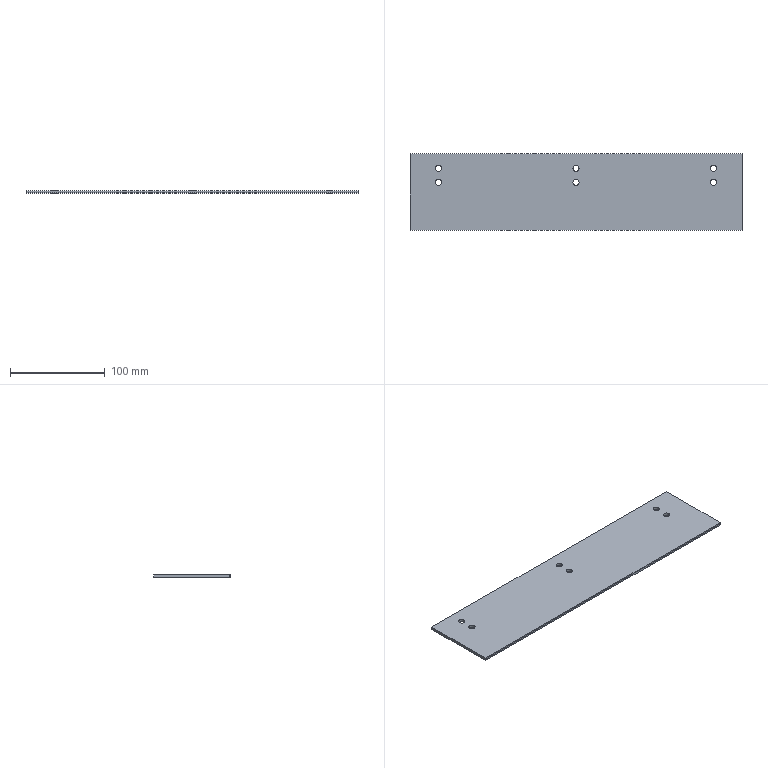Part | SolidWorks | features Extrusion 1, ICE 1 | 1 solid | 19 faces | box 350 x 80.217 x 3 mm | volume 83584 mm3 | cylinder 14 | plane 5 | commonest cylinder face diameters 6.5 x12 33.7 x2
STEP:
#1=CARTESIAN_POINT('',(-175.,-37.65,1.5));
#2=VERTEX_POINT('',#1);
#3=CARTESIAN_POINT('',(-175.,-37.717,3.));
#4=VERTEX_POINT('',#3);
#5=CARTESIAN_POINT('',(-175.,-54.5,1.5));
#6=DIRECTION('',(1.,0.,0.));
#7=DIRECTION('',(0.,0.,-1.));
#8=AXIS2_PLACEMENT_3D('',#5,#6,#7);
#9=CIRCLE('',#8,16.85);
#10=EDGE_CURVE('',#2,#4,#9,.T.);
#11=ORIENTED_EDGE('',*,*,#10,.F.);
#12=CARTESIAN_POINT('',(175.,-37.65,1.5));
#13=VERTEX_POINT('',#12);
#14=CARTESIAN_POINT('',(-191.,-37.65,1.5));
#15=DIRECTION('',(1.,0.,0.));
#16=VECTOR('',#15,1000.);
#17=LINE('',#14,#16);
#18=EDGE_CURVE('',#2,#13,#17,.T.);
#19=ORIENTED_EDGE('',*,*,#18,.T.);
#20=CARTESIAN_POINT('',(175.,-37.717,3.));
#21=VERTEX_POINT('',#20);
#22=CARTESIAN_POINT('',(175.,-54.5,1.5));
#23=DIRECTION('',(1.,0.,0.));
#24=DIRECTION('',(0.,1.,0.));
#25=AXIS2_PLACEMENT_3D('',#22,#23,#24);
#26=CIRCLE('',#25,16.85);
#27=EDGE_CURVE('',#13,#21,#26,.T.);
#28=ORIENTED_EDGE('',*,*,#27,.T.);
#29=CARTESIAN_POINT('',(-191.,-37.717,3.));
#30=DIRECTION('',(-1.,0.,0.));
#31=VECTOR('',#30,1000.);
#32=LINE('',#29,#31);
#33=EDGE_CURVE('',#21,#4,#32,.T.);
#34=ORIENTED_EDGE('',*,*,#33,.T.);
#35=EDGE_LOOP('',(#11,#19,#28,#34));
#36=FACE_OUTER_BOUND('',#35,.T.);
#37=CARTESIAN_POINT('',(-191.,-54.5,1.5));
#38=DIRECTION('',(1.,0.,0.));
#39=DIRECTION('',(0.,1.,0.));
#40=AXIS2_PLACEMENT_3D('',#37,#38,#39);
#41=CYLINDRICAL_SURFACE('',#40,16.85);
#42=ADVANCED_FACE('',(#36),#41,.F.);
#43=CARTESIAN_POINT('',(141.75,12.5,3.));
#44=VERTEX_POINT('',#43);
#45=CARTESIAN_POINT('',(148.25,12.5,3.));
#46=VERTEX_POINT('',#45);
#47=CARTESIAN_POINT('',(145.,12.5,3.));
#48=DIRECTION('',(0.,0.,1.));
#49=DIRECTION('',(1.,0.,0.));
#50=AXIS2_PLACEMENT_3D('',#47,#48,#49);
#51=CIRCLE('',#50,3.25);
#52=EDGE_CURVE('',#44,#46,#51,.T.);
#53=ORIENTED_EDGE('',*,*,#52,.T.);
#54=CARTESIAN_POINT('',(148.25,12.5,0.));
#55=VERTEX_POINT('',#54);
#56=CARTESIAN_POINT('',(148.25,12.5,3.));
#57=DIRECTION('',(0.,0.,-1.));
#58=VECTOR('',#57,1000.);
#59=LINE('',#56,#58);
#60=EDGE_CURVE('',#46,#55,#59,.T.);
#61=ORIENTED_EDGE('',*,*,#60,.T.);
#62=CARTESIAN_POINT('',(141.75,12.5,0.));
#63=VERTEX_POINT('',#62);
#64=CARTESIAN_POINT('',(145.,12.5,0.));
#65=DIRECTION('',(0.,0.,1.));
#66=DIRECTION('',(1.,0.,0.));
#67=AXIS2_PLACEMENT_3D('',#64,#65,#66);
#68=CIRCLE('',#67,3.25);
#69=EDGE_CURVE('',#63,#55,#68,.T.);
#70=ORIENTED_EDGE('',*,*,#69,.F.);
#71=CARTESIAN_POINT('',(141.75,12.5,3.));
#72=DIRECTION('',(0.,0.,-1.));
#73=VECTOR('',#72,1000.);
#74=LINE('',#71,#73);
#75=EDGE_CURVE('',#44,#63,#74,.T.);
#76=ORIENTED_EDGE('',*,*,#75,.F.);
#77=EDGE_LOOP('',(#53,#61,#70,#76));
#78=FACE_OUTER_BOUND('',#77,.T.);
#79=CARTESIAN_POINT('',(145.,12.5,3.));
#80=DIRECTION('',(0.,0.,-1.));
#81=DIRECTION('',(-1.,0.,0.));
#82=AXIS2_PLACEMENT_3D('',#79,#80,#81);
#83=CYLINDRICAL_SURFACE('',#82,3.25);
#84=ADVANCED_FACE('',(#78),#83,.F.);
#85=CARTESIAN_POINT('',(141.75,27.5,3.));
#86=VERTEX_POINT('',#85);
#87=CARTESIAN_POINT('',(148.25,27.5,3.));
#88=VERTEX_POINT('',#87);
#89=CARTESIAN_POINT('',(145.,27.5,3.));
#90=DIRECTION('',(0.,0.,1.));
#91=DIRECTION('',(1.,0.,0.));
#92=AXIS2_PLACEMENT_3D('',#89,#90,#91);
#93=CIRCLE('',#92,3.25);
#94=EDGE_CURVE('',#86,#88,#93,.T.);
#95=ORIENTED_EDGE('',*,*,#94,.T.);
#96=CARTESIAN_POINT('',(148.25,27.5,0.));
#97=VERTEX_POINT('',#96);
#98=CARTESIAN_POINT('',(148.25,27.5,3.));
#99=DIRECTION('',(0.,0.,-1.));
#100=VECTOR('',#99,1000.);
#101=LINE('',#98,#100);
#102=EDGE_CURVE('',#88,#97,#101,.T.);
#103=ORIENTED_EDGE('',*,*,#102,.T.);
#104=CARTESIAN_POINT('',(141.75,27.5,0.));
#105=VERTEX_POINT('',#104);
#106=CARTESIAN_POINT('',(145.,27.5,0.));
#107=DIRECTION('',(0.,0.,1.));
#108=DIRECTION('',(1.,0.,0.));
#109=AXIS2_PLACEMENT_3D('',#106,#107,#108);
#110=CIRCLE('',#109,3.25);
#111=EDGE_CURVE('',#105,#97,#110,.T.);
#112=ORIENTED_EDGE('',*,*,#111,.F.);
#113=CARTESIAN_POINT('',(141.75,27.5,3.));
#114=DIRECTION('',(0.,0.,-1.));
#115=VECTOR('',#114,1000.);
#116=LINE('',#113,#115);
#117=EDGE_CURVE('',#86,#105,#116,.T.);
#118=ORIENTED_EDGE('',*,*,#117,.F.);
#119=EDGE_LOOP('',(#95,#103,#112,#118));
#120=FACE_OUTER_BOUND('',#119,.T.);
#121=CARTESIAN_POINT('',(145.,27.5,3.));
#122=DIRECTION('',(0.,0.,-1.));
#123=DIRECTION('',(-1.,0.,0.));
#124=AXIS2_PLACEMENT_3D('',#121,#122,#123);
#125=CYLINDRICAL_SURFACE('',#124,3.25);
#126=ADVANCED_FACE('',(#120),#125,.F.);
#127=CARTESIAN_POINT('',(-3.25,12.5,3.));
#128=VERTEX_POINT('',#127);
#129=CARTESIAN_POINT('',(3.25,12.5,3.));
#130=VERTEX_POINT('',#129);
#131=CARTESIAN_POINT('',(0.,12.5,3.));
#132=DIRECTION('',(0.,0.,1.));
#133=DIRECTION('',(1.,0.,0.));
#134=AXIS2_PLACEMENT_3D('',#131,#132,#133);
#135=CIRCLE('',#134,3.25);
#136=EDGE_CURVE('',#128,#130,#135,.T.);
#137=ORIENTED_EDGE('',*,*,#136,.T.);
#138=CARTESIAN_POINT('',(3.25,12.5,0.));
#139=VERTEX_POINT('',#138);
#140=CARTESIAN_POINT('',(3.25,12.5,3.));
#141=DIRECTION('',(0.,0.,-1.));
#142=VECTOR('',#141,1000.);
#143=LINE('',#140,#142);
#144=EDGE_CURVE('',#130,#139,#143,.T.);
#145=ORIENTED_EDGE('',*,*,#144,.T.);
#146=CARTESIAN_POINT('',(-3.25,12.5,0.));
#147=VERTEX_POINT('',#146);
#148=CARTESIAN_POINT('',(0.,12.5,0.));
#149=DIRECTION('',(0.,0.,1.));
#150=DIRECTION('',(1.,0.,0.));
#151=AXIS2_PLACEMENT_3D('',#148,#149,#150);
#152=CIRCLE('',#151,3.25);
#153=EDGE_CURVE('',#147,#139,#152,.T.);
#154=ORIENTED_EDGE('',*,*,#153,.F.);
#155=CARTESIAN_POINT('',(-3.25,12.5,3.));
#156=DIRECTION('',(0.,0.,-1.));
#157=VECTOR('',#156,1000.);
#158=LINE('',#155,#157);
#159=EDGE_CURVE('',#128,#147,#158,.T.);
#160=ORIENTED_EDGE('',*,*,#159,.F.);
#161=EDGE_LOOP('',(#137,#145,#154,#160));
#162=FACE_OUTER_BOUND('',#161,.T.);
#163=CARTESIAN_POINT('',(0.,12.5,3.));
#164=DIRECTION('',(0.,0.,-1.));
#165=DIRECTION('',(-1.,0.,0.));
#166=AXIS2_PLACEMENT_3D('',#163,#164,#165);
#167=CYLINDRICAL_SURFACE('',#166,3.25);
#168=ADVANCED_FACE('',(#162),#167,.F.);
#169=CARTESIAN_POINT('',(-3.25,27.5,3.));
#170=VERTEX_POINT('',#169);
#171=CARTESIAN_POINT('',(3.25,27.5,3.));
#172=VERTEX_POINT('',#171);
#173=CARTESIAN_POINT('',(0.,27.5,3.));
#174=DIRECTION('',(0.,0.,1.));
#175=DIRECTION('',(1.,0.,0.));
#176=AXIS2_PLACEMENT_3D('',#173,#174,#175);
#177=CIRCLE('',#176,3.25);
#178=EDGE_CURVE('',#170,#172,#177,.T.);
#179=ORIENTED_EDGE('',*,*,#178,.T.);
#180=CARTESIAN_POINT('',(3.25,27.5,0.));
#181=VERTEX_POINT('',#180);
#182=CARTESIAN_POINT('',(3.25,27.5,3.));
#183=DIRECTION('',(0.,0.,-1.));
#184=VECTOR('',#183,1000.);
#185=LINE('',#182,#184);
#186=EDGE_CURVE('',#172,#181,#185,.T.);
#187=ORIENTED_EDGE('',*,*,#186,.T.);
#188=CARTESIAN_POINT('',(-3.25,27.5,0.));
#189=VERTEX_POINT('',#188);
#190=CARTESIAN_POINT('',(0.,27.5,0.));
#191=DIRECTION('',(0.,0.,1.));
#192=DIRECTION('',(1.,0.,0.));
#193=AXIS2_PLACEMENT_3D('',#190,#191,#192);
#194=CIRCLE('',#193,3.25);
#195=EDGE_CURVE('',#189,#181,#194,.T.);
#196=ORIENTED_EDGE('',*,*,#195,.F.);
#197=CARTESIAN_POINT('',(-3.25,27.5,3.));
#198=DIRECTION('',(0.,0.,-1.));
#199=VECTOR('',#198,1000.);
#200=LINE('',#197,#199);
#201=EDGE_CURVE('',#170,#189,#200,.T.);
#202=ORIENTED_EDGE('',*,*,#201,.F.);
#203=EDGE_LOOP('',(#179,#187,#196,#202));
#204=FACE_OUTER_BOUND('',#203,.T.);
#205=CARTESIAN_POINT('',(0.,27.5,3.));
#206=DIRECTION('',(0.,0.,-1.));
#207=DIRECTION('',(-1.,0.,0.));
#208=AXIS2_PLACEMENT_3D('',#205,#206,#207);
#209=CYLINDRICAL_SURFACE('',#208,3.25);
#210=ADVANCED_FACE('',(#204),#209,.F.);
#211=CARTESIAN_POINT('',(-148.25,12.5,3.));
#212=VERTEX_POINT('',#211);
#213=CARTESIAN_POINT('',(-141.75,12.5,3.));
#214=VERTEX_POINT('',#213);
#215=CARTESIAN_POINT('',(-145.,12.5,3.));
#216=DIRECTION('',(0.,0.,1.));
#217=DIRECTION('',(1.,0.,0.));
#218=AXIS2_PLACEMENT_3D('',#215,#216,#217);
#219=CIRCLE('',#218,3.25);
#220=EDGE_CURVE('',#212,#214,#219,.T.);
#221=ORIENTED_EDGE('',*,*,#220,.T.);
#222=CARTESIAN_POINT('',(-141.75,12.5,0.));
#223=VERTEX_POINT('',#222);
#224=CARTESIAN_POINT('',(-141.75,12.5,3.));
#225=DIRECTION('',(0.,0.,-1.));
#226=VECTOR('',#225,1000.);
#227=LINE('',#224,#226);
#228=EDGE_CURVE('',#214,#223,#227,.T.);
#229=ORIENTED_EDGE('',*,*,#228,.T.);
#230=CARTESIAN_POINT('',(-148.25,12.5,0.));
#231=VERTEX_POINT('',#230);
#232=CARTESIAN_POINT('',(-145.,12.5,0.));
#233=DIRECTION('',(0.,0.,1.));
#234=DIRECTION('',(1.,0.,0.));
#235=AXIS2_PLACEMENT_3D('',#232,#233,#234);
#236=CIRCLE('',#235,3.25);
#237=EDGE_CURVE('',#231,#223,#236,.T.);
#238=ORIENTED_EDGE('',*,*,#237,.F.);
#239=CARTESIAN_POINT('',(-148.25,12.5,3.));
#240=DIRECTION('',(0.,0.,-1.));
#241=VECTOR('',#240,1000.);
#242=LINE('',#239,#241);
#243=EDGE_CURVE('',#212,#231,#242,.T.);
#244=ORIENTED_EDGE('',*,*,#243,.F.);
#245=EDGE_LOOP('',(#221,#229,#238,#244));
#246=FACE_OUTER_BOUND('',#245,.T.);
#247=CARTESIAN_POINT('',(-145.,12.5,3.));
#248=DIRECTION('',(0.,0.,-1.));
#249=DIRECTION('',(-1.,0.,0.));
#250=AXIS2_PLACEMENT_3D('',#247,#248,#249);
#251=CYLINDRICAL_SURFACE('',#250,3.25);
#252=ADVANCED_FACE('',(#246),#251,.F.);
#253=CARTESIAN_POINT('',(-148.25,27.5,3.));
#254=VERTEX_POINT('',#253);
#255=CARTESIAN_POINT('',(-141.75,27.5,3.));
#256=VERTEX_POINT('',#255);
#257=CARTESIAN_POINT('',(-145.,27.5,3.));
#258=DIRECTION('',(0.,0.,1.));
#259=DIRECTION('',(1.,0.,0.));
#260=AXIS2_PLACEMENT_3D('',#257,#258,#259);
#261=CIRCLE('',#260,3.25);
#262=EDGE_CURVE('',#254,#256,#261,.T.);
#263=ORIENTED_EDGE('',*,*,#262,.T.);
#264=CARTESIAN_POINT('',(-141.75,27.5,0.));
#265=VERTEX_POINT('',#264);
#266=CARTESIAN_POINT('',(-141.75,27.5,3.));
#267=DIRECTION('',(0.,0.,-1.));
#268=VECTOR('',#267,1000.);
#269=LINE('',#266,#268);
#270=EDGE_CURVE('',#256,#265,#269,.T.);
#271=ORIENTED_EDGE('',*,*,#270,.T.);
#272=CARTESIAN_POINT('',(-148.25,27.5,0.));
#273=VERTEX_POINT('',#272);
#274=CARTESIAN_POINT('',(-145.,27.5,0.));
#275=DIRECTION('',(0.,0.,1.));
#276=DIRECTION('',(1.,0.,0.));
#277=AXIS2_PLACEMENT_3D('',#274,#275,#276);
#278=CIRCLE('',#277,3.25);
#279=EDGE_CURVE('',#273,#265,#278,.T.);
#280=ORIENTED_EDGE('',*,*,#279,.F.);
#281=CARTESIAN_POINT('',(-148.25,27.5,3.));
#282=DIRECTION('',(0.,0.,-1.));
#283=VECTOR('',#282,1000.);
#284=LINE('',#281,#283);
#285=EDGE_CURVE('',#254,#273,#284,.T.);
#286=ORIENTED_EDGE('',*,*,#285,.F.);
#287=EDGE_LOOP('',(#263,#271,#280,#286));
#288=FACE_OUTER_BOUND('',#287,.T.);
#289=CARTESIAN_POINT('',(-145.,27.5,3.));
#290=DIRECTION('',(0.,0.,-1.));
#291=DIRECTION('',(-1.,0.,0.));
#292=AXIS2_PLACEMENT_3D('',#289,#290,#291);
#293=CYLINDRICAL_SURFACE('',#292,3.25);
#294=ADVANCED_FACE('',(#288),#293,.F.);
#295=ORIENTED_EDGE('',*,*,#33,.F.);
#296=CARTESIAN_POINT('',(175.,42.5,3.));
#297=VERTEX_POINT('',#296);
#298=CARTESIAN_POINT('',(175.,42.5,3.));
#299=DIRECTION('',(0.,1.,0.));
#300=VECTOR('',#299,1000.);
#301=LINE('',#298,#300);
#302=EDGE_CURVE('',#21,#297,#301,.T.);
#303=ORIENTED_EDGE('',*,*,#302,.T.);
#304=CARTESIAN_POINT('',(-175.,42.5,3.));
#305=VERTEX_POINT('',#304);
#306=CARTESIAN_POINT('',(-175.,42.5,3.));
#307=DIRECTION('',(-1.,0.,0.));
#308=VECTOR('',#307,1000.);
#309=LINE('',#306,#308);
#310=EDGE_CURVE('',#297,#305,#309,.T.);
#311=ORIENTED_EDGE('',*,*,#310,.T.);
#312=CARTESIAN_POINT('',(-175.,42.5,3.));
#313=DIRECTION('',(0.,-1.,0.));
#314=VECTOR('',#313,1000.);
#315=LINE('',#312,#314);
#316=EDGE_CURVE('',#305,#4,#315,.T.);
#317=ORIENTED_EDGE('',*,*,#316,.T.);
#318=EDGE_LOOP('',(#295,#303,#311,#317));
#319=FACE_OUTER_BOUND('',#318,.T.);
#320=ORIENTED_EDGE('',*,*,#94,.F.);
#321=CARTESIAN_POINT('',(145.,27.5,3.));
#322=DIRECTION('',(0.,0.,1.));
#323=DIRECTION('',(1.,0.,0.));
#324=AXIS2_PLACEMENT_3D('',#321,#322,#323);
#325=CIRCLE('',#324,3.25);
#326=EDGE_CURVE('',#88,#86,#325,.T.);
#327=ORIENTED_EDGE('',*,*,#326,.F.);
#328=EDGE_LOOP('',(#320,#327));
#329=FACE_BOUND('',#328,.T.);
#330=ORIENTED_EDGE('',*,*,#178,.F.);
#331=CARTESIAN_POINT('',(0.,27.5,3.));
#332=DIRECTION('',(0.,0.,1.));
#333=DIRECTION('',(1.,0.,0.));
#334=AXIS2_PLACEMENT_3D('',#331,#332,#333);
#335=CIRCLE('',#334,3.25);
#336=EDGE_CURVE('',#172,#170,#335,.T.);
#337=ORIENTED_EDGE('',*,*,#336,.F.);
#338=EDGE_LOOP('',(#330,#337));
#339=FACE_BOUND('',#338,.T.);
#340=ORIENTED_EDGE('',*,*,#262,.F.);
#341=CARTESIAN_POINT('',(-145.,27.5,3.));
#342=DIRECTION('',(0.,0.,1.));
#343=DIRECTION('',(1.,0.,0.));
#344=AXIS2_PLACEMENT_3D('',#341,#342,#343);
#345=CIRCLE('',#344,3.25);
#346=EDGE_CURVE('',#256,#254,#345,.T.);
#347=ORIENTED_EDGE('',*,*,#346,.F.);
#348=EDGE_LOOP('',(#340,#347));
#349=FACE_BOUND('',#348,.T.);
#350=ORIENTED_EDGE('',*,*,#220,.F.);
#351=CARTESIAN_POINT('',(-145.,12.5,3.));
#352=DIRECTION('',(0.,0.,1.));
#353=DIRECTION('',(1.,0.,0.));
#354=AXIS2_PLACEMENT_3D('',#351,#352,#353);
#355=CIRCLE('',#354,3.25);
#356=EDGE_CURVE('',#214,#212,#355,.T.);
#357=ORIENTED_EDGE('',*,*,#356,.F.);
#358=EDGE_LOOP('',(#350,#357));
#359=FACE_BOUND('',#358,.T.);
#360=ORIENTED_EDGE('',*,*,#136,.F.);
#361=CARTESIAN_POINT('',(0.,12.5,3.));
#362=DIRECTION('',(0.,0.,1.));
#363=DIRECTION('',(1.,0.,0.));
#364=AXIS2_PLACEMENT_3D('',#361,#362,#363);
#365=CIRCLE('',#364,3.25);
#366=EDGE_CURVE('',#130,#128,#365,.T.);
#367=ORIENTED_EDGE('',*,*,#366,.F.);
#368=EDGE_LOOP('',(#360,#367));
#369=FACE_BOUND('',#368,.T.);
#370=ORIENTED_EDGE('',*,*,#52,.F.);
#371=CARTESIAN_POINT('',(145.,12.5,3.));
#372=DIRECTION('',(0.,0.,1.));
#373=DIRECTION('',(1.,0.,0.));
#374=AXIS2_PLACEMENT_3D('',#371,#372,#373);
#375=CIRCLE('',#374,3.25);
#376=EDGE_CURVE('',#46,#44,#375,.T.);
#377=ORIENTED_EDGE('',*,*,#376,.F.);
#378=EDGE_LOOP('',(#370,#377));
#379=FACE_BOUND('',#378,.T.);
#380=CARTESIAN_POINT('',(0.,0.,3.));
#381=DIRECTION('',(0.,0.,1.));
#382=DIRECTION('',(1.,0.,0.));
#383=AXIS2_PLACEMENT_3D('',#380,#381,#382);
#384=PLANE('',#383);
#385=ADVANCED_FACE('',(#319,#329,#339,#349,#359,#369,#379),#384,.T.);
#386=CARTESIAN_POINT('',(175.,-37.717,0.));
#387=VERTEX_POINT('',#386);
#388=CARTESIAN_POINT('',(175.,42.5,0.));
#389=VERTEX_POINT('',#388);
#390=CARTESIAN_POINT('',(175.,42.5,0.));
#391=DIRECTION('',(0.,1.,0.));
#392=VECTOR('',#391,1000.);
#393=LINE('',#390,#392);
#394=EDGE_CURVE('',#387,#389,#393,.T.);
#395=ORIENTED_EDGE('',*,*,#394,.F.);
#396=CARTESIAN_POINT('',(-175.,-37.717,0.));
#397=VERTEX_POINT('',#396);
#398=CARTESIAN_POINT('',(-191.,-37.717,0.));
#399=DIRECTION('',(-1.,0.,0.));
#400=VECTOR('',#399,1000.);
#401=LINE('',#398,#400);
#402=EDGE_CURVE('',#387,#397,#401,.T.);
#403=ORIENTED_EDGE('',*,*,#402,.T.);
#404=CARTESIAN_POINT('',(-175.,42.5,0.));
#405=VERTEX_POINT('',#404);
#406=CARTESIAN_POINT('',(-175.,42.5,0.));
#407=DIRECTION('',(0.,-1.,0.));
#408=VECTOR('',#407,1000.);
#409=LINE('',#406,#408);
#410=EDGE_CURVE('',#405,#397,#409,.T.);
#411=ORIENTED_EDGE('',*,*,#410,.F.);
#412=CARTESIAN_POINT('',(-175.,42.5,0.));
#413=DIRECTION('',(-1.,0.,0.));
#414=VECTOR('',#413,1000.);
#415=LINE('',#412,#414);
#416=EDGE_CURVE('',#389,#405,#415,.T.);
#417=ORIENTED_EDGE('',*,*,#416,.F.);
#418=EDGE_LOOP('',(#395,#403,#411,#417));
#419=FACE_OUTER_BOUND('',#418,.T.);
#420=ORIENTED_EDGE('',*,*,#279,.T.);
#421=CARTESIAN_POINT('',(-145.,27.5,0.));
#422=DIRECTION('',(0.,0.,1.));
#423=DIRECTION('',(1.,0.,0.));
#424=AXIS2_PLACEMENT_3D('',#421,#422,#423);
#425=CIRCLE('',#424,3.25);
#426=EDGE_CURVE('',#265,#273,#425,.T.);
#427=ORIENTED_EDGE('',*,*,#426,.T.);
#428=EDGE_LOOP('',(#420,#427));
#429=FACE_BOUND('',#428,.T.);
#430=ORIENTED_EDGE('',*,*,#237,.T.);
#431=CARTESIAN_POINT('',(-145.,12.5,0.));
#432=DIRECTION('',(0.,0.,1.));
#433=DIRECTION('',(1.,0.,0.));
#434=AXIS2_PLACEMENT_3D('',#431,#432,#433);
#435=CIRCLE('',#434,3.25);
#436=EDGE_CURVE('',#223,#231,#435,.T.);
#437=ORIENTED_EDGE('',*,*,#436,.T.);
#438=EDGE_LOOP('',(#430,#437));
#439=FACE_BOUND('',#438,.T.);
#440=ORIENTED_EDGE('',*,*,#195,.T.);
#441=CARTESIAN_POINT('',(0.,27.5,0.));
#442=DIRECTION('',(0.,0.,1.));
#443=DIRECTION('',(1.,0.,0.));
#444=AXIS2_PLACEMENT_3D('',#441,#442,#443);
#445=CIRCLE('',#444,3.25);
#446=EDGE_CURVE('',#181,#189,#445,.T.);
#447=ORIENTED_EDGE('',*,*,#446,.T.);
#448=EDGE_LOOP('',(#440,#447));
#449=FACE_BOUND('',#448,.T.);
#450=ORIENTED_EDGE('',*,*,#153,.T.);
#451=CARTESIAN_POINT('',(0.,12.5,0.));
#452=DIRECTION('',(0.,0.,1.));
#453=DIRECTION('',(1.,0.,0.));
#454=AXIS2_PLACEMENT_3D('',#451,#452,#453);
#455=CIRCLE('',#454,3.25);
#456=EDGE_CURVE('',#139,#147,#455,.T.);
#457=ORIENTED_EDGE('',*,*,#456,.T.);
#458=EDGE_LOOP('',(#450,#457));
#459=FACE_BOUND('',#458,.T.);
#460=ORIENTED_EDGE('',*,*,#111,.T.);
#461=CARTESIAN_POINT('',(145.,27.5,0.));
#462=DIRECTION('',(0.,0.,1.));
#463=DIRECTION('',(1.,0.,0.));
#464=AXIS2_PLACEMENT_3D('',#461,#462,#463);
#465=CIRCLE('',#464,3.25);
#466=EDGE_CURVE('',#97,#105,#465,.T.);
#467=ORIENTED_EDGE('',*,*,#466,.T.);
#468=EDGE_LOOP('',(#460,#467));
#469=FACE_BOUND('',#468,.T.);
#470=ORIENTED_EDGE('',*,*,#69,.T.);
#471=CARTESIAN_POINT('',(145.,12.5,0.));
#472=DIRECTION('',(0.,0.,1.));
#473=DIRECTION('',(1.,0.,0.));
#474=AXIS2_PLACEMENT_3D('',#471,#472,#473);
#475=CIRCLE('',#474,3.25);
#476=EDGE_CURVE('',#55,#63,#475,.T.);
#477=ORIENTED_EDGE('',*,*,#476,.T.);
#478=EDGE_LOOP('',(#470,#477));
#479=FACE_BOUND('',#478,.T.);
#480=CARTESIAN_POINT('',(0.,0.,0.));
#481=DIRECTION('',(0.,0.,1.));
#482=DIRECTION('',(1.,0.,0.));
#483=AXIS2_PLACEMENT_3D('',#480,#481,#482);
#484=PLANE('',#483);
#485=ADVANCED_FACE('',(#419,#429,#439,#449,#459,#469,#479),#484,.F.);
#486=ORIENTED_EDGE('',*,*,#302,.F.);
#487=ORIENTED_EDGE('',*,*,#27,.F.);
#488=CARTESIAN_POINT('',(175.,-54.5,1.5));
#489=DIRECTION('',(1.,0.,0.));
#490=DIRECTION('',(0.,1.,0.));
#491=AXIS2_PLACEMENT_3D('',#488,#489,#490);
#492=CIRCLE('',#491,16.85);
#493=EDGE_CURVE('',#387,#13,#492,.T.);
#494=ORIENTED_EDGE('',*,*,#493,.F.);
#495=ORIENTED_EDGE('',*,*,#394,.T.);
#496=CARTESIAN_POINT('',(175.,42.5,3.));
#497=DIRECTION('',(0.,0.,-1.));
#498=VECTOR('',#497,1000.);
#499=LINE('',#496,#498);
#500=EDGE_CURVE('',#297,#389,#499,.T.);
#501=ORIENTED_EDGE('',*,*,#500,.F.);
#502=EDGE_LOOP('',(#486,#487,#494,#495,#501));
#503=FACE_OUTER_BOUND('',#502,.T.);
#504=CARTESIAN_POINT('',(175.,42.5,3.));
#505=DIRECTION('',(-1.,0.,0.));
#506=DIRECTION('',(0.,-1.,0.));
#507=AXIS2_PLACEMENT_3D('',#504,#505,#506);
#508=PLANE('',#507);
#509=ADVANCED_FACE('',(#503),#508,.F.);
#510=ORIENTED_EDGE('',*,*,#416,.T.);
#511=CARTESIAN_POINT('',(-175.,42.5,3.));
#512=DIRECTION('',(0.,0.,-1.));
#513=VECTOR('',#512,1000.);
#514=LINE('',#511,#513);
#515=EDGE_CURVE('',#305,#405,#514,.T.);
#516=ORIENTED_EDGE('',*,*,#515,.F.);
#517=ORIENTED_EDGE('',*,*,#310,.F.);
#518=ORIENTED_EDGE('',*,*,#500,.T.);
#519=EDGE_LOOP('',(#510,#516,#517,#518));
#520=FACE_OUTER_BOUND('',#519,.T.);
#521=CARTESIAN_POINT('',(-175.,42.5,3.));
#522=DIRECTION('',(0.,-1.,0.));
#523=DIRECTION('',(0.,0.,-1.));
#524=AXIS2_PLACEMENT_3D('',#521,#522,#523);
#525=PLANE('',#524);
#526=ADVANCED_FACE('',(#520),#525,.F.);
#527=ORIENTED_EDGE('',*,*,#410,.T.);
#528=CARTESIAN_POINT('',(-175.,-54.5,1.5));
#529=DIRECTION('',(1.,0.,0.));
#530=DIRECTION('',(0.,0.,-1.));
#531=AXIS2_PLACEMENT_3D('',#528,#529,#530);
#532=CIRCLE('',#531,16.85);
#533=EDGE_CURVE('',#397,#2,#532,.T.);
#534=ORIENTED_EDGE('',*,*,#533,.T.);
#535=ORIENTED_EDGE('',*,*,#10,.T.);
#536=ORIENTED_EDGE('',*,*,#316,.F.);
#537=ORIENTED_EDGE('',*,*,#515,.T.);
#538=EDGE_LOOP('',(#527,#534,#535,#536,#537));
#539=FACE_OUTER_BOUND('',#538,.T.);
#540=CARTESIAN_POINT('',(-175.,42.5,3.));
#541=DIRECTION('',(1.,0.,0.));
#542=DIRECTION('',(0.,0.,-1.));
#543=AXIS2_PLACEMENT_3D('',#540,#541,#542);
#544=PLANE('',#543);
#545=ADVANCED_FACE('',(#539),#544,.F.);
#546=ORIENTED_EDGE('',*,*,#270,.F.);
#547=ORIENTED_EDGE('',*,*,#346,.T.);
#548=ORIENTED_EDGE('',*,*,#285,.T.);
#549=ORIENTED_EDGE('',*,*,#426,.F.);
#550=EDGE_LOOP('',(#546,#547,#548,#549));
#551=FACE_OUTER_BOUND('',#550,.T.);
#552=CARTESIAN_POINT('',(-145.,27.5,3.));
#553=DIRECTION('',(0.,0.,-1.));
#554=DIRECTION('',(-1.,0.,0.));
#555=AXIS2_PLACEMENT_3D('',#552,#553,#554);
#556=CYLINDRICAL_SURFACE('',#555,3.25);
#557=ADVANCED_FACE('',(#551),#556,.F.);
#558=ORIENTED_EDGE('',*,*,#228,.F.);
#559=ORIENTED_EDGE('',*,*,#356,.T.);
#560=ORIENTED_EDGE('',*,*,#243,.T.);
#561=ORIENTED_EDGE('',*,*,#436,.F.);
#562=EDGE_LOOP('',(#558,#559,#560,#561));
#563=FACE_OUTER_BOUND('',#562,.T.);
#564=CARTESIAN_POINT('',(-145.,12.5,3.));
#565=DIRECTION('',(0.,0.,-1.));
#566=DIRECTION('',(-1.,0.,0.));
#567=AXIS2_PLACEMENT_3D('',#564,#565,#566);
#568=CYLINDRICAL_SURFACE('',#567,3.25);
#569=ADVANCED_FACE('',(#563),#568,.F.);
#570=ORIENTED_EDGE('',*,*,#186,.F.);
#571=ORIENTED_EDGE('',*,*,#336,.T.);
#572=ORIENTED_EDGE('',*,*,#201,.T.);
#573=ORIENTED_EDGE('',*,*,#446,.F.);
#574=EDGE_LOOP('',(#570,#571,#572,#573));
#575=FACE_OUTER_BOUND('',#574,.T.);
#576=CARTESIAN_POINT('',(0.,27.5,3.));
#577=DIRECTION('',(0.,0.,-1.));
#578=DIRECTION('',(-1.,0.,0.));
#579=AXIS2_PLACEMENT_3D('',#576,#577,#578);
#580=CYLINDRICAL_SURFACE('',#579,3.25);
#581=ADVANCED_FACE('',(#575),#580,.F.);
#582=ORIENTED_EDGE('',*,*,#144,.F.);
#583=ORIENTED_EDGE('',*,*,#366,.T.);
#584=ORIENTED_EDGE('',*,*,#159,.T.);
#585=ORIENTED_EDGE('',*,*,#456,.F.);
#586=EDGE_LOOP('',(#582,#583,#584,#585));
#587=FACE_OUTER_BOUND('',#586,.T.);
#588=CARTESIAN_POINT('',(0.,12.5,3.));
#589=DIRECTION('',(0.,0.,-1.));
#590=DIRECTION('',(-1.,0.,0.));
#591=AXIS2_PLACEMENT_3D('',#588,#589,#590);
#592=CYLINDRICAL_SURFACE('',#591,3.25);
#593=ADVANCED_FACE('',(#587),#592,.F.);
#594=ORIENTED_EDGE('',*,*,#102,.F.);
#595=ORIENTED_EDGE('',*,*,#326,.T.);
#596=ORIENTED_EDGE('',*,*,#117,.T.);
#597=ORIENTED_EDGE('',*,*,#466,.F.);
#598=EDGE_LOOP('',(#594,#595,#596,#597));
#599=FACE_OUTER_BOUND('',#598,.T.);
#600=CARTESIAN_POINT('',(145.,27.5,3.));
#601=DIRECTION('',(0.,0.,-1.));
#602=DIRECTION('',(-1.,0.,0.));
#603=AXIS2_PLACEMENT_3D('',#600,#601,#602);
#604=CYLINDRICAL_SURFACE('',#603,3.25);
#605=ADVANCED_FACE('',(#599),#604,.F.);
#606=ORIENTED_EDGE('',*,*,#60,.F.);
#607=ORIENTED_EDGE('',*,*,#376,.T.);
#608=ORIENTED_EDGE('',*,*,#75,.T.);
#609=ORIENTED_EDGE('',*,*,#476,.F.);
#610=EDGE_LOOP('',(#606,#607,#608,#609));
#611=FACE_OUTER_BOUND('',#610,.T.);
#612=CARTESIAN_POINT('',(145.,12.5,3.));
#613=DIRECTION('',(0.,0.,-1.));
#614=DIRECTION('',(-1.,0.,0.));
#615=AXIS2_PLACEMENT_3D('',#612,#613,#614);
#616=CYLINDRICAL_SURFACE('',#615,3.25);
#617=ADVANCED_FACE('',(#611),#616,.F.);
#618=ORIENTED_EDGE('',*,*,#18,.F.);
#619=ORIENTED_EDGE('',*,*,#533,.F.);
#620=ORIENTED_EDGE('',*,*,#402,.F.);
#621=ORIENTED_EDGE('',*,*,#493,.T.);
#622=EDGE_LOOP('',(#618,#619,#620,#621));
#623=FACE_OUTER_BOUND('',#622,.T.);
#624=CARTESIAN_POINT('',(-191.,-54.5,1.5));
#625=DIRECTION('',(1.,0.,0.));
#626=DIRECTION('',(0.,1.,0.));
#627=AXIS2_PLACEMENT_3D('',#624,#625,#626);
#628=CYLINDRICAL_SURFACE('',#627,16.85);
#629=ADVANCED_FACE('',(#623),#628,.F.);
#630=CLOSED_SHELL('',(#42,#84,#126,#168,#210,#252,#294,#385,#485,#509,#526,#545,#557,#569,#581,#593,#605,#617,#629));
#631=MANIFOLD_SOLID_BREP('',#630);
#632=CARTESIAN_POINT('',(0.,0.,0.));
#633=DIRECTION('',(0.,0.,1.));
#634=DIRECTION('',(1.,0.,0.));
#635=AXIS2_PLACEMENT_3D('',#632,#633,#634);
#636=(LENGTH_UNIT()NAMED_UNIT(*)SI_UNIT(.MILLI.,.METRE.));
#637=UNCERTAINTY_MEASURE_WITH_UNIT(LENGTH_MEASURE(0.00001),#636,'','');
#638=(NAMED_UNIT(*)PLANE_ANGLE_UNIT()SI_UNIT($,.RADIAN.));
#639=(NAMED_UNIT(*)SI_UNIT($,.STERADIAN.)SOLID_ANGLE_UNIT());
#640=(GEOMETRIC_REPRESENTATION_CONTEXT(3)GLOBAL_UNCERTAINTY_ASSIGNED_CONTEXT((#637))GLOBAL_UNIT_ASSIGNED_CONTEXT((#636,#638,#639))REPRESENTATION_CONTEXT('',''));
#641=ADVANCED_BREP_SHAPE_REPRESENTATION('',(#631,#635),#640);